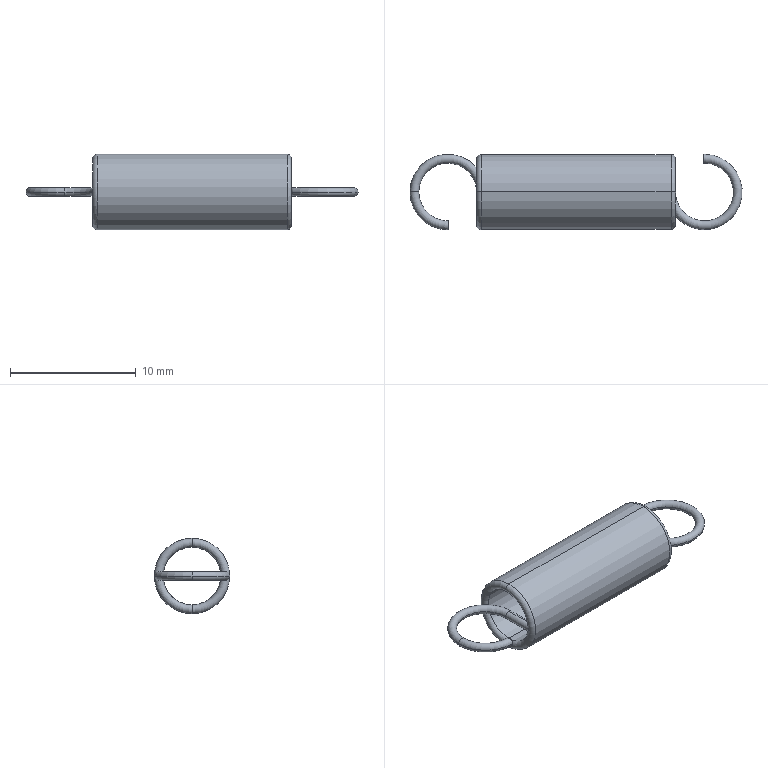Part | STEP file | QA-AWU6_25 | 1 solid | 20 faces | box 26.4 x 6 x 6 mm | volume 193.836 mm3 | torus 10 | cylinder 8 | plane 2 | commonest cylinder face diameters 0.7 x4 4.6 x2 6 x2